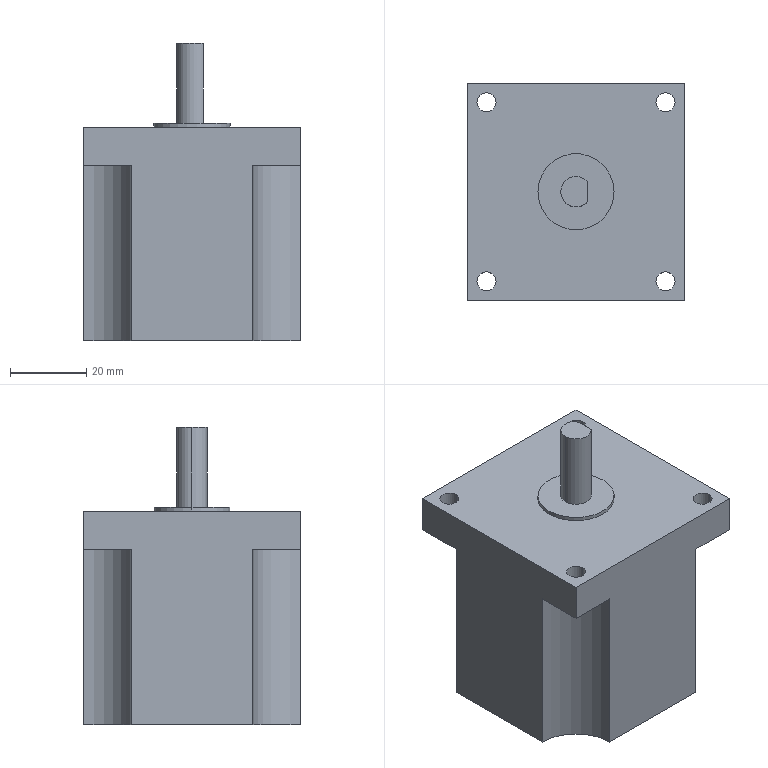Part | SolidWorks | features ICE 5, Extrusion 1 | 1 solid | 29 faces | box 57 x 57 x 78 mm | volume 159872 mm3 | cylinder 16 | plane 13 | commonest cylinder face diameters 5 x8 25 x4 8 x2 20 x2
STEP:
#1=CARTESIAN_POINT('',(-4.,0.,78.));
#2=VERTEX_POINT('',#1);
#3=CARTESIAN_POINT('',(3.,-2.646,78.));
#4=VERTEX_POINT('',#3);
#5=CARTESIAN_POINT('',(0.,0.,78.));
#6=DIRECTION('',(0.,0.,1.));
#7=DIRECTION('',(1.,0.,0.));
#8=AXIS2_PLACEMENT_3D('',#5,#6,#7);
#9=CIRCLE('',#8,4.);
#10=EDGE_CURVE('',#2,#4,#9,.T.);
#11=ORIENTED_EDGE('',*,*,#10,.F.);
#12=CARTESIAN_POINT('',(-4.,0.,57.));
#13=VERTEX_POINT('',#12);
#14=CARTESIAN_POINT('',(-4.,0.,78.));
#15=DIRECTION('',(0.,0.,-1.));
#16=VECTOR('',#15,1000.);
#17=LINE('',#14,#16);
#18=EDGE_CURVE('',#2,#13,#17,.T.);
#19=ORIENTED_EDGE('',*,*,#18,.T.);
#20=CARTESIAN_POINT('',(3.,-2.646,57.));
#21=VERTEX_POINT('',#20);
#22=CARTESIAN_POINT('',(0.,0.,57.));
#23=DIRECTION('',(0.,0.,1.));
#24=DIRECTION('',(1.,0.,0.));
#25=AXIS2_PLACEMENT_3D('',#22,#23,#24);
#26=CIRCLE('',#25,4.);
#27=EDGE_CURVE('',#13,#21,#26,.T.);
#28=ORIENTED_EDGE('',*,*,#27,.T.);
#29=CARTESIAN_POINT('',(3.,-2.646,57.));
#30=DIRECTION('',(0.,0.,1.));
#31=VECTOR('',#30,1000.);
#32=LINE('',#29,#31);
#33=EDGE_CURVE('',#21,#4,#32,.T.);
#34=ORIENTED_EDGE('',*,*,#33,.T.);
#35=EDGE_LOOP('',(#11,#19,#28,#34));
#36=FACE_OUTER_BOUND('',#35,.T.);
#37=CARTESIAN_POINT('',(0.,0.,78.));
#38=DIRECTION('',(0.,0.,-1.));
#39=DIRECTION('',(-1.,0.,0.));
#40=AXIS2_PLACEMENT_3D('',#37,#38,#39);
#41=CYLINDRICAL_SURFACE('',#40,4.);
#42=ADVANCED_FACE('',(#36),#41,.T.);
#43=CARTESIAN_POINT('',(10.,0.,57.));
#44=VERTEX_POINT('',#43);
#45=CARTESIAN_POINT('',(-10.,0.,57.));
#46=VERTEX_POINT('',#45);
#47=CARTESIAN_POINT('',(0.,0.,57.));
#48=DIRECTION('',(0.,0.,1.));
#49=DIRECTION('',(1.,0.,0.));
#50=AXIS2_PLACEMENT_3D('',#47,#48,#49);
#51=CIRCLE('',#50,10.);
#52=EDGE_CURVE('',#44,#46,#51,.T.);
#53=ORIENTED_EDGE('',*,*,#52,.F.);
#54=CARTESIAN_POINT('',(10.,0.,56.));
#55=VERTEX_POINT('',#54);
#56=CARTESIAN_POINT('',(10.,0.,57.));
#57=DIRECTION('',(0.,0.,-1.));
#58=VECTOR('',#57,1000.);
#59=LINE('',#56,#58);
#60=EDGE_CURVE('',#44,#55,#59,.T.);
#61=ORIENTED_EDGE('',*,*,#60,.T.);
#62=CARTESIAN_POINT('',(-10.,0.,56.));
#63=VERTEX_POINT('',#62);
#64=CARTESIAN_POINT('',(0.,0.,56.));
#65=DIRECTION('',(0.,0.,1.));
#66=DIRECTION('',(1.,0.,0.));
#67=AXIS2_PLACEMENT_3D('',#64,#65,#66);
#68=CIRCLE('',#67,10.);
#69=EDGE_CURVE('',#55,#63,#68,.T.);
#70=ORIENTED_EDGE('',*,*,#69,.T.);
#71=CARTESIAN_POINT('',(-10.,0.,57.));
#72=DIRECTION('',(0.,0.,-1.));
#73=VECTOR('',#72,1000.);
#74=LINE('',#71,#73);
#75=EDGE_CURVE('',#46,#63,#74,.T.);
#76=ORIENTED_EDGE('',*,*,#75,.F.);
#77=EDGE_LOOP('',(#53,#61,#70,#76));
#78=FACE_OUTER_BOUND('',#77,.T.);
#79=CARTESIAN_POINT('',(0.,0.,57.));
#80=DIRECTION('',(0.,0.,-1.));
#81=DIRECTION('',(-1.,0.,0.));
#82=AXIS2_PLACEMENT_3D('',#79,#80,#81);
#83=CYLINDRICAL_SURFACE('',#82,10.);
#84=ADVANCED_FACE('',(#78),#83,.T.);
#85=CARTESIAN_POINT('',(-21.,-23.5,46.));
#86=VERTEX_POINT('',#85);
#87=CARTESIAN_POINT('',(-26.,-23.5,46.));
#88=VERTEX_POINT('',#87);
#89=CARTESIAN_POINT('',(-23.5,-23.5,46.));
#90=DIRECTION('',(0.,0.,-1.));
#91=DIRECTION('',(1.,0.,0.));
#92=AXIS2_PLACEMENT_3D('',#89,#90,#91);
#93=CIRCLE('',#92,2.5);
#94=EDGE_CURVE('',#86,#88,#93,.T.);
#95=ORIENTED_EDGE('',*,*,#94,.T.);
#96=CARTESIAN_POINT('',(-26.,-23.5,56.));
#97=VERTEX_POINT('',#96);
#98=CARTESIAN_POINT('',(-26.,-23.5,-42.));
#99=DIRECTION('',(0.,0.,1.));
#100=VECTOR('',#99,1000.);
#101=LINE('',#98,#100);
#102=EDGE_CURVE('',#88,#97,#101,.T.);
#103=ORIENTED_EDGE('',*,*,#102,.T.);
#104=CARTESIAN_POINT('',(-21.,-23.5,56.));
#105=VERTEX_POINT('',#104);
#106=CARTESIAN_POINT('',(-23.5,-23.5,56.));
#107=DIRECTION('',(0.,0.,1.));
#108=DIRECTION('',(1.,0.,0.));
#109=AXIS2_PLACEMENT_3D('',#106,#107,#108);
#110=CIRCLE('',#109,2.5);
#111=EDGE_CURVE('',#97,#105,#110,.T.);
#112=ORIENTED_EDGE('',*,*,#111,.T.);
#113=CARTESIAN_POINT('',(-21.,-23.5,-42.));
#114=DIRECTION('',(0.,0.,1.));
#115=VECTOR('',#114,1000.);
#116=LINE('',#113,#115);
#117=EDGE_CURVE('',#86,#105,#116,.T.);
#118=ORIENTED_EDGE('',*,*,#117,.F.);
#119=EDGE_LOOP('',(#95,#103,#112,#118));
#120=FACE_OUTER_BOUND('',#119,.T.);
#121=CARTESIAN_POINT('',(-23.5,-23.5,-42.));
#122=DIRECTION('',(0.,0.,1.));
#123=DIRECTION('',(1.,0.,0.));
#124=AXIS2_PLACEMENT_3D('',#121,#122,#123);
#125=CYLINDRICAL_SURFACE('',#124,2.5);
#126=ADVANCED_FACE('',(#120),#125,.F.);
#127=CARTESIAN_POINT('',(26.,-23.5,46.));
#128=VERTEX_POINT('',#127);
#129=CARTESIAN_POINT('',(21.,-23.5,46.));
#130=VERTEX_POINT('',#129);
#131=CARTESIAN_POINT('',(23.5,-23.5,46.));
#132=DIRECTION('',(0.,0.,-1.));
#133=DIRECTION('',(1.,0.,0.));
#134=AXIS2_PLACEMENT_3D('',#131,#132,#133);
#135=CIRCLE('',#134,2.5);
#136=EDGE_CURVE('',#128,#130,#135,.T.);
#137=ORIENTED_EDGE('',*,*,#136,.T.);
#138=CARTESIAN_POINT('',(21.,-23.5,56.));
#139=VERTEX_POINT('',#138);
#140=CARTESIAN_POINT('',(21.,-23.5,-42.));
#141=DIRECTION('',(0.,0.,1.));
#142=VECTOR('',#141,1000.);
#143=LINE('',#140,#142);
#144=EDGE_CURVE('',#130,#139,#143,.T.);
#145=ORIENTED_EDGE('',*,*,#144,.T.);
#146=CARTESIAN_POINT('',(26.,-23.5,56.));
#147=VERTEX_POINT('',#146);
#148=CARTESIAN_POINT('',(23.5,-23.5,56.));
#149=DIRECTION('',(0.,0.,1.));
#150=DIRECTION('',(1.,0.,0.));
#151=AXIS2_PLACEMENT_3D('',#148,#149,#150);
#152=CIRCLE('',#151,2.5);
#153=EDGE_CURVE('',#139,#147,#152,.T.);
#154=ORIENTED_EDGE('',*,*,#153,.T.);
#155=CARTESIAN_POINT('',(26.,-23.5,-42.));
#156=DIRECTION('',(0.,0.,1.));
#157=VECTOR('',#156,1000.);
#158=LINE('',#155,#157);
#159=EDGE_CURVE('',#128,#147,#158,.T.);
#160=ORIENTED_EDGE('',*,*,#159,.F.);
#161=EDGE_LOOP('',(#137,#145,#154,#160));
#162=FACE_OUTER_BOUND('',#161,.T.);
#163=CARTESIAN_POINT('',(23.5,-23.5,-42.));
#164=DIRECTION('',(0.,0.,1.));
#165=DIRECTION('',(1.,0.,0.));
#166=AXIS2_PLACEMENT_3D('',#163,#164,#165);
#167=CYLINDRICAL_SURFACE('',#166,2.5);
#168=ADVANCED_FACE('',(#162),#167,.F.);
#169=CARTESIAN_POINT('',(26.,23.5,46.));
#170=VERTEX_POINT('',#169);
#171=CARTESIAN_POINT('',(21.,23.5,46.));
#172=VERTEX_POINT('',#171);
#173=CARTESIAN_POINT('',(23.5,23.5,46.));
#174=DIRECTION('',(0.,0.,-1.));
#175=DIRECTION('',(1.,0.,0.));
#176=AXIS2_PLACEMENT_3D('',#173,#174,#175);
#177=CIRCLE('',#176,2.5);
#178=EDGE_CURVE('',#170,#172,#177,.T.);
#179=ORIENTED_EDGE('',*,*,#178,.T.);
#180=CARTESIAN_POINT('',(21.,23.5,56.));
#181=VERTEX_POINT('',#180);
#182=CARTESIAN_POINT('',(21.,23.5,-42.));
#183=DIRECTION('',(0.,0.,1.));
#184=VECTOR('',#183,1000.);
#185=LINE('',#182,#184);
#186=EDGE_CURVE('',#172,#181,#185,.T.);
#187=ORIENTED_EDGE('',*,*,#186,.T.);
#188=CARTESIAN_POINT('',(26.,23.5,56.));
#189=VERTEX_POINT('',#188);
#190=CARTESIAN_POINT('',(23.5,23.5,56.));
#191=DIRECTION('',(0.,0.,1.));
#192=DIRECTION('',(1.,0.,0.));
#193=AXIS2_PLACEMENT_3D('',#190,#191,#192);
#194=CIRCLE('',#193,2.5);
#195=EDGE_CURVE('',#181,#189,#194,.T.);
#196=ORIENTED_EDGE('',*,*,#195,.T.);
#197=CARTESIAN_POINT('',(26.,23.5,-42.));
#198=DIRECTION('',(0.,0.,1.));
#199=VECTOR('',#198,1000.);
#200=LINE('',#197,#199);
#201=EDGE_CURVE('',#170,#189,#200,.T.);
#202=ORIENTED_EDGE('',*,*,#201,.F.);
#203=EDGE_LOOP('',(#179,#187,#196,#202));
#204=FACE_OUTER_BOUND('',#203,.T.);
#205=CARTESIAN_POINT('',(23.5,23.5,-42.));
#206=DIRECTION('',(0.,0.,1.));
#207=DIRECTION('',(1.,0.,0.));
#208=AXIS2_PLACEMENT_3D('',#205,#206,#207);
#209=CYLINDRICAL_SURFACE('',#208,2.5);
#210=ADVANCED_FACE('',(#204),#209,.F.);
#211=CARTESIAN_POINT('',(-21.,23.5,46.));
#212=VERTEX_POINT('',#211);
#213=CARTESIAN_POINT('',(-26.,23.5,46.));
#214=VERTEX_POINT('',#213);
#215=CARTESIAN_POINT('',(-23.5,23.5,46.));
#216=DIRECTION('',(0.,0.,-1.));
#217=DIRECTION('',(1.,0.,0.));
#218=AXIS2_PLACEMENT_3D('',#215,#216,#217);
#219=CIRCLE('',#218,2.5);
#220=EDGE_CURVE('',#212,#214,#219,.T.);
#221=ORIENTED_EDGE('',*,*,#220,.T.);
#222=CARTESIAN_POINT('',(-26.,23.5,56.));
#223=VERTEX_POINT('',#222);
#224=CARTESIAN_POINT('',(-26.,23.5,-42.));
#225=DIRECTION('',(0.,0.,1.));
#226=VECTOR('',#225,1000.);
#227=LINE('',#224,#226);
#228=EDGE_CURVE('',#214,#223,#227,.T.);
#229=ORIENTED_EDGE('',*,*,#228,.T.);
#230=CARTESIAN_POINT('',(-21.,23.5,56.));
#231=VERTEX_POINT('',#230);
#232=CARTESIAN_POINT('',(-23.5,23.5,56.));
#233=DIRECTION('',(0.,0.,1.));
#234=DIRECTION('',(1.,0.,0.));
#235=AXIS2_PLACEMENT_3D('',#232,#233,#234);
#236=CIRCLE('',#235,2.5);
#237=EDGE_CURVE('',#223,#231,#236,.T.);
#238=ORIENTED_EDGE('',*,*,#237,.T.);
#239=CARTESIAN_POINT('',(-21.,23.5,-42.));
#240=DIRECTION('',(0.,0.,1.));
#241=VECTOR('',#240,1000.);
#242=LINE('',#239,#241);
#243=EDGE_CURVE('',#212,#231,#242,.T.);
#244=ORIENTED_EDGE('',*,*,#243,.F.);
#245=EDGE_LOOP('',(#221,#229,#238,#244));
#246=FACE_OUTER_BOUND('',#245,.T.);
#247=CARTESIAN_POINT('',(-23.5,23.5,-42.));
#248=DIRECTION('',(0.,0.,1.));
#249=DIRECTION('',(1.,0.,0.));
#250=AXIS2_PLACEMENT_3D('',#247,#248,#249);
#251=CYLINDRICAL_SURFACE('',#250,2.5);
#252=ADVANCED_FACE('',(#246),#251,.F.);
#253=CARTESIAN_POINT('',(-28.5,-16.,0.));
#254=VERTEX_POINT('',#253);
#255=CARTESIAN_POINT('',(-28.5,-16.,46.));
#256=VERTEX_POINT('',#255);
#257=CARTESIAN_POINT('',(-28.5,-16.,91.355));
#258=DIRECTION('',(0.,0.,1.));
#259=VECTOR('',#258,1000.);
#260=LINE('',#257,#259);
#261=EDGE_CURVE('',#254,#256,#260,.T.);
#262=ORIENTED_EDGE('',*,*,#261,.T.);
#263=CARTESIAN_POINT('',(-28.5,-28.5,46.));
#264=VERTEX_POINT('',#263);
#265=CARTESIAN_POINT('',(-28.5,-28.5,46.));
#266=DIRECTION('',(0.,-1.,0.));
#267=VECTOR('',#266,1000.);
#268=LINE('',#265,#267);
#269=EDGE_CURVE('',#256,#264,#268,.T.);
#270=ORIENTED_EDGE('',*,*,#269,.T.);
#271=CARTESIAN_POINT('',(-28.5,-28.5,56.));
#272=VERTEX_POINT('',#271);
#273=CARTESIAN_POINT('',(-28.5,-28.5,56.));
#274=DIRECTION('',(0.,0.,-1.));
#275=VECTOR('',#274,1000.);
#276=LINE('',#273,#275);
#277=EDGE_CURVE('',#272,#264,#276,.T.);
#278=ORIENTED_EDGE('',*,*,#277,.F.);
#279=CARTESIAN_POINT('',(-28.5,28.5,56.));
#280=VERTEX_POINT('',#279);
#281=CARTESIAN_POINT('',(-28.5,-28.5,56.));
#282=DIRECTION('',(0.,-1.,0.));
#283=VECTOR('',#282,1000.);
#284=LINE('',#281,#283);
#285=EDGE_CURVE('',#280,#272,#284,.T.);
#286=ORIENTED_EDGE('',*,*,#285,.F.);
#287=CARTESIAN_POINT('',(-28.5,28.5,46.));
#288=VERTEX_POINT('',#287);
#289=CARTESIAN_POINT('',(-28.5,28.5,56.));
#290=DIRECTION('',(0.,0.,-1.));
#291=VECTOR('',#290,1000.);
#292=LINE('',#289,#291);
#293=EDGE_CURVE('',#280,#288,#292,.T.);
#294=ORIENTED_EDGE('',*,*,#293,.T.);
#295=CARTESIAN_POINT('',(-28.5,16.,46.));
#296=VERTEX_POINT('',#295);
#297=CARTESIAN_POINT('',(-28.5,-28.5,46.));
#298=DIRECTION('',(0.,-1.,0.));
#299=VECTOR('',#298,1000.);
#300=LINE('',#297,#299);
#301=EDGE_CURVE('',#288,#296,#300,.T.);
#302=ORIENTED_EDGE('',*,*,#301,.T.);
#303=CARTESIAN_POINT('',(-28.5,16.,0.));
#304=VERTEX_POINT('',#303);
#305=CARTESIAN_POINT('',(-28.5,16.,91.355));
#306=DIRECTION('',(0.,0.,-1.));
#307=VECTOR('',#306,1000.);
#308=LINE('',#305,#307);
#309=EDGE_CURVE('',#296,#304,#308,.T.);
#310=ORIENTED_EDGE('',*,*,#309,.T.);
#311=CARTESIAN_POINT('',(-28.5,-28.5,0.));
#312=DIRECTION('',(0.,-1.,0.));
#313=VECTOR('',#312,1000.);
#314=LINE('',#311,#313);
#315=EDGE_CURVE('',#304,#254,#314,.T.);
#316=ORIENTED_EDGE('',*,*,#315,.T.);
#317=EDGE_LOOP('',(#262,#270,#278,#286,#294,#302,#310,#316));
#318=FACE_OUTER_BOUND('',#317,.T.);
#319=CARTESIAN_POINT('',(-28.5,-28.5,56.));
#320=DIRECTION('',(1.,0.,0.));
#321=DIRECTION('',(0.,0.,-1.));
#322=AXIS2_PLACEMENT_3D('',#319,#320,#321);
#323=PLANE('',#322);
#324=ADVANCED_FACE('',(#318),#323,.F.);
#325=CARTESIAN_POINT('',(16.,-28.5,0.));
#326=VERTEX_POINT('',#325);
#327=CARTESIAN_POINT('',(16.,-28.5,46.));
#328=VERTEX_POINT('',#327);
#329=CARTESIAN_POINT('',(16.,-28.5,91.355));
#330=DIRECTION('',(0.,0.,1.));
#331=VECTOR('',#330,1000.);
#332=LINE('',#329,#331);
#333=EDGE_CURVE('',#326,#328,#332,.T.);
#334=ORIENTED_EDGE('',*,*,#333,.T.);
#335=CARTESIAN_POINT('',(28.5,-28.5,46.));
#336=VERTEX_POINT('',#335);
#337=CARTESIAN_POINT('',(28.5,-28.5,46.));
#338=DIRECTION('',(1.,0.,0.));
#339=VECTOR('',#338,1000.);
#340=LINE('',#337,#339);
#341=EDGE_CURVE('',#328,#336,#340,.T.);
#342=ORIENTED_EDGE('',*,*,#341,.T.);
#343=CARTESIAN_POINT('',(28.5,-28.5,56.));
#344=VERTEX_POINT('',#343);
#345=CARTESIAN_POINT('',(28.5,-28.5,56.));
#346=DIRECTION('',(0.,0.,-1.));
#347=VECTOR('',#346,1000.);
#348=LINE('',#345,#347);
#349=EDGE_CURVE('',#344,#336,#348,.T.);
#350=ORIENTED_EDGE('',*,*,#349,.F.);
#351=CARTESIAN_POINT('',(28.5,-28.5,56.));
#352=DIRECTION('',(1.,0.,0.));
#353=VECTOR('',#352,1000.);
#354=LINE('',#351,#353);
#355=EDGE_CURVE('',#272,#344,#354,.T.);
#356=ORIENTED_EDGE('',*,*,#355,.F.);
#357=ORIENTED_EDGE('',*,*,#277,.T.);
#358=CARTESIAN_POINT('',(-16.,-28.5,46.));
#359=VERTEX_POINT('',#358);
#360=CARTESIAN_POINT('',(28.5,-28.5,46.));
#361=DIRECTION('',(1.,0.,0.));
#362=VECTOR('',#361,1000.);
#363=LINE('',#360,#362);
#364=EDGE_CURVE('',#264,#359,#363,.T.);
#365=ORIENTED_EDGE('',*,*,#364,.T.);
#366=CARTESIAN_POINT('',(-16.,-28.5,0.));
#367=VERTEX_POINT('',#366);
#368=CARTESIAN_POINT('',(-16.,-28.5,91.355));
#369=DIRECTION('',(0.,0.,-1.));
#370=VECTOR('',#369,1000.);
#371=LINE('',#368,#370);
#372=EDGE_CURVE('',#359,#367,#371,.T.);
#373=ORIENTED_EDGE('',*,*,#372,.T.);
#374=CARTESIAN_POINT('',(28.5,-28.5,0.));
#375=DIRECTION('',(1.,0.,0.));
#376=VECTOR('',#375,1000.);
#377=LINE('',#374,#376);
#378=EDGE_CURVE('',#367,#326,#377,.T.);
#379=ORIENTED_EDGE('',*,*,#378,.T.);
#380=EDGE_LOOP('',(#334,#342,#350,#356,#357,#365,#373,#379));
#381=FACE_OUTER_BOUND('',#380,.T.);
#382=CARTESIAN_POINT('',(28.5,-28.5,56.));
#383=DIRECTION('',(0.,1.,0.));
#384=DIRECTION('',(-1.,0.,0.));
#385=AXIS2_PLACEMENT_3D('',#382,#383,#384);
#386=PLANE('',#385);
#387=ADVANCED_FACE('',(#381),#386,.F.);
#388=ORIENTED_EDGE('',*,*,#349,.T.);
#389=CARTESIAN_POINT('',(28.5,-16.,46.));
#390=VERTEX_POINT('',#389);
#391=CARTESIAN_POINT('',(28.5,-28.5,46.));
#392=DIRECTION('',(0.,1.,0.));
#393=VECTOR('',#392,1000.);
#394=LINE('',#391,#393);
#395=EDGE_CURVE('',#336,#390,#394,.T.);
#396=ORIENTED_EDGE('',*,*,#395,.T.);
#397=CARTESIAN_POINT('',(28.5,-16.,0.));
#398=VERTEX_POINT('',#397);
#399=CARTESIAN_POINT('',(28.5,-16.,91.355));
#400=DIRECTION('',(0.,0.,-1.));
#401=VECTOR('',#400,1000.);
#402=LINE('',#399,#401);
#403=EDGE_CURVE('',#390,#398,#402,.T.);
#404=ORIENTED_EDGE('',*,*,#403,.T.);
#405=CARTESIAN_POINT('',(28.5,16.,0.));
#406=VERTEX_POINT('',#405);
#407=CARTESIAN_POINT('',(28.5,-28.5,0.));
#408=DIRECTION('',(0.,1.,0.));
#409=VECTOR('',#408,1000.);
#410=LINE('',#407,#409);
#411=EDGE_CURVE('',#398,#406,#410,.T.);
#412=ORIENTED_EDGE('',*,*,#411,.T.);
#413=CARTESIAN_POINT('',(28.5,16.,46.));
#414=VERTEX_POINT('',#413);
#415=CARTESIAN_POINT('',(28.5,16.,91.355));
#416=DIRECTION('',(0.,0.,1.));
#417=VECTOR('',#416,1000.);
#418=LINE('',#415,#417);
#419=EDGE_CURVE('',#406,#414,#418,.T.);
#420=ORIENTED_EDGE('',*,*,#419,.T.);
#421=CARTESIAN_POINT('',(28.5,28.5,46.));
#422=VERTEX_POINT('',#421);
#423=CARTESIAN_POINT('',(28.5,-28.5,46.));
#424=DIRECTION('',(0.,1.,0.));
#425=VECTOR('',#424,1000.);
#426=LINE('',#423,#425);
#427=EDGE_CURVE('',#414,#422,#426,.T.);
#428=ORIENTED_EDGE('',*,*,#427,.T.);
#429=CARTESIAN_POINT('',(28.5,28.5,56.));
#430=VERTEX_POINT('',#429);
#431=CARTESIAN_POINT('',(28.5,28.5,56.));
#432=DIRECTION('',(0.,0.,-1.));
#433=VECTOR('',#432,1000.);
#434=LINE('',#431,#433);
#435=EDGE_CURVE('',#430,#422,#434,.T.);
#436=ORIENTED_EDGE('',*,*,#435,.F.);
#437=CARTESIAN_POINT('',(28.5,-28.5,56.));
#438=DIRECTION('',(0.,1.,0.));
#439=VECTOR('',#438,1000.);
#440=LINE('',#437,#439);
#441=EDGE_CURVE('',#344,#430,#440,.T.);
#442=ORIENTED_EDGE('',*,*,#441,.F.);
#443=EDGE_LOOP('',(#388,#396,#404,#412,#420,#428,#436,#442));
#444=FACE_OUTER_BOUND('',#443,.T.);
#445=CARTESIAN_POINT('',(28.5,-28.5,56.));
#446=DIRECTION('',(-1.,0.,0.));
#447=DIRECTION('',(0.,0.,1.));
#448=AXIS2_PLACEMENT_3D('',#445,#446,#447);
#449=PLANE('',#448);
#450=ADVANCED_FACE('',(#444),#449,.F.);
#451=CARTESIAN_POINT('',(-16.,28.5,0.));
#452=VERTEX_POINT('',#451);
#453=CARTESIAN_POINT('',(-16.,28.5,46.));
#454=VERTEX_POINT('',#453);
#455=CARTESIAN_POINT('',(-16.,28.5,91.355));
#456=DIRECTION('',(0.,0.,1.));
#457=VECTOR('',#456,1000.);
#458=LINE('',#455,#457);
#459=EDGE_CURVE('',#452,#454,#458,.T.);
#460=ORIENTED_EDGE('',*,*,#459,.T.);
#461=CARTESIAN_POINT('',(28.5,28.5,46.));
#462=DIRECTION('',(-1.,0.,0.));
#463=VECTOR('',#462,1000.);
#464=LINE('',#461,#463);
#465=EDGE_CURVE('',#454,#288,#464,.T.);
#466=ORIENTED_EDGE('',*,*,#465,.T.);
#467=ORIENTED_EDGE('',*,*,#293,.F.);
#468=CARTESIAN_POINT('',(28.5,28.5,56.));
#469=DIRECTION('',(-1.,0.,0.));
#470=VECTOR('',#469,1000.);
#471=LINE('',#468,#470);
#472=EDGE_CURVE('',#430,#280,#471,.T.);
#473=ORIENTED_EDGE('',*,*,#472,.F.);
#474=ORIENTED_EDGE('',*,*,#435,.T.);
#475=CARTESIAN_POINT('',(16.,28.5,46.));
#476=VERTEX_POINT('',#475);
#477=CARTESIAN_POINT('',(28.5,28.5,46.));
#478=DIRECTION('',(-1.,0.,0.));
#479=VECTOR('',#478,1000.);
#480=LINE('',#477,#479);
#481=EDGE_CURVE('',#422,#476,#480,.T.);
#482=ORIENTED_EDGE('',*,*,#481,.T.);
#483=CARTESIAN_POINT('',(16.,28.5,0.));
#484=VERTEX_POINT('',#483);
#485=CARTESIAN_POINT('',(16.,28.5,91.355));
#486=DIRECTION('',(0.,0.,-1.));
#487=VECTOR('',#486,1000.);
#488=LINE('',#485,#487);
#489=EDGE_CURVE('',#476,#484,#488,.T.);
#490=ORIENTED_EDGE('',*,*,#489,.T.);
#491=CARTESIAN_POINT('',(28.5,28.5,0.));
#492=DIRECTION('',(-1.,0.,0.));
#493=VECTOR('',#492,1000.);
#494=LINE('',#491,#493);
#495=EDGE_CURVE('',#484,#452,#494,.T.);
#496=ORIENTED_EDGE('',*,*,#495,.T.);
#497=EDGE_LOOP('',(#460,#466,#467,#473,#474,#482,#490,#496));
#498=FACE_OUTER_BOUND('',#497,.T.);
#499=CARTESIAN_POINT('',(28.5,28.5,56.));
#500=DIRECTION('',(0.,-1.,0.));
#501=DIRECTION('',(1.,0.,0.));
#502=AXIS2_PLACEMENT_3D('',#499,#500,#501);
#503=PLANE('',#502);
#504=ADVANCED_FACE('',(#498),#503,.F.);
#505=CARTESIAN_POINT('',(0.,0.,56.));
#506=DIRECTION('',(0.,0.,1.));
#507=DIRECTION('',(1.,0.,0.));
#508=AXIS2_PLACEMENT_3D('',#505,#506,#507);
#509=CIRCLE('',#508,10.);
#510=EDGE_CURVE('',#63,#55,#509,.T.);
#511=ORIENTED_EDGE('',*,*,#510,.F.);
#512=ORIENTED_EDGE('',*,*,#69,.F.);
#513=EDGE_LOOP('',(#511,#512));
#514=FACE_BOUND('',#513,.T.);
#515=CARTESIAN_POINT('',(-23.5,-23.5,56.));
#516=DIRECTION('',(0.,0.,1.));
#517=DIRECTION('',(1.,0.,0.));
#518=AXIS2_PLACEMENT_3D('',#515,#516,#517);
#519=CIRCLE('',#518,2.5);
#520=EDGE_CURVE('',#105,#97,#519,.T.);
#521=ORIENTED_EDGE('',*,*,#520,.F.);
#522=ORIENTED_EDGE('',*,*,#111,.F.);
#523=EDGE_LOOP('',(#521,#522));
#524=FACE_BOUND('',#523,.T.);
#525=CARTESIAN_POINT('',(23.5,-23.5,56.));
#526=DIRECTION('',(0.,0.,1.));
#527=DIRECTION('',(1.,0.,0.));
#528=AXIS2_PLACEMENT_3D('',#525,#526,#527);
#529=CIRCLE('',#528,2.5);
#530=EDGE_CURVE('',#147,#139,#529,.T.);
#531=ORIENTED_EDGE('',*,*,#530,.F.);
#532=ORIENTED_EDGE('',*,*,#153,.F.);
#533=EDGE_LOOP('',(#531,#532));
#534=FACE_BOUND('',#533,.T.);
#535=CARTESIAN_POINT('',(23.5,23.5,56.));
#536=DIRECTION('',(0.,0.,1.));
#537=DIRECTION('',(1.,0.,0.));
#538=AXIS2_PLACEMENT_3D('',#535,#536,#537);
#539=CIRCLE('',#538,2.5);
#540=EDGE_CURVE('',#189,#181,#539,.T.);
#541=ORIENTED_EDGE('',*,*,#540,.F.);
#542=ORIENTED_EDGE('',*,*,#195,.F.);
#543=EDGE_LOOP('',(#541,#542));
#544=FACE_BOUND('',#543,.T.);
#545=CARTESIAN_POINT('',(-23.5,23.5,56.));
#546=DIRECTION('',(0.,0.,1.));
#547=DIRECTION('',(1.,0.,0.));
#548=AXIS2_PLACEMENT_3D('',#545,#546,#547);
#549=CIRCLE('',#548,2.5);
#550=EDGE_CURVE('',#231,#223,#549,.T.);
#551=ORIENTED_EDGE('',*,*,#550,.F.);
#552=ORIENTED_EDGE('',*,*,#237,.F.);
#553=EDGE_LOOP('',(#551,#552));
#554=FACE_BOUND('',#553,.T.);
#555=ORIENTED_EDGE('',*,*,#285,.T.);
#556=ORIENTED_EDGE('',*,*,#355,.T.);
#557=ORIENTED_EDGE('',*,*,#441,.T.);
#558=ORIENTED_EDGE('',*,*,#472,.T.);
#559=EDGE_LOOP('',(#555,#556,#557,#558));
#560=FACE_OUTER_BOUND('',#559,.T.);
#561=CARTESIAN_POINT('',(0.,0.,56.));
#562=DIRECTION('',(0.,0.,1.));
#563=DIRECTION('',(1.,0.,0.));
#564=AXIS2_PLACEMENT_3D('',#561,#562,#563);
#565=PLANE('',#564);
#566=ADVANCED_FACE('',(#514,#524,#534,#544,#554,#560),#565,.T.);
#567=ORIENTED_EDGE('',*,*,#411,.F.);
#568=CARTESIAN_POINT('',(28.5,-28.5,0.));
#569=DIRECTION('',(0.,0.,-1.));
#570=DIRECTION('',(-1.,0.,0.));
#571=AXIS2_PLACEMENT_3D('',#568,#569,#570);
#572=CIRCLE('',#571,12.5);
#573=EDGE_CURVE('',#326,#398,#572,.T.);
#574=ORIENTED_EDGE('',*,*,#573,.F.);
#575=ORIENTED_EDGE('',*,*,#378,.F.);
#576=CARTESIAN_POINT('',(-28.5,-28.5,0.));
#577=DIRECTION('',(0.,0.,-1.));
#578=DIRECTION('',(-1.,0.,0.));
#579=AXIS2_PLACEMENT_3D('',#576,#577,#578);
#580=CIRCLE('',#579,12.5);
#581=EDGE_CURVE('',#254,#367,#580,.T.);
#582=ORIENTED_EDGE('',*,*,#581,.F.);
#583=ORIENTED_EDGE('',*,*,#315,.F.);
#584=CARTESIAN_POINT('',(-28.5,28.5,0.));
#585=DIRECTION('',(0.,0.,-1.));
#586=DIRECTION('',(-1.,0.,0.));
#587=AXIS2_PLACEMENT_3D('',#584,#585,#586);
#588=CIRCLE('',#587,12.5);
#589=EDGE_CURVE('',#452,#304,#588,.T.);
#590=ORIENTED_EDGE('',*,*,#589,.F.);
#591=ORIENTED_EDGE('',*,*,#495,.F.);
#592=CARTESIAN_POINT('',(28.5,28.5,0.));
#593=DIRECTION('',(0.,0.,-1.));
#594=DIRECTION('',(-1.,0.,0.));
#595=AXIS2_PLACEMENT_3D('',#592,#593,#594);
#596=CIRCLE('',#595,12.5);
#597=EDGE_CURVE('',#406,#484,#596,.T.);
#598=ORIENTED_EDGE('',*,*,#597,.F.);
#599=EDGE_LOOP('',(#567,#574,#575,#582,#583,#590,#591,#598));
#600=FACE_OUTER_BOUND('',#599,.T.);
#601=CARTESIAN_POINT('',(0.,0.,0.));
#602=DIRECTION('',(0.,0.,1.));
#603=DIRECTION('',(1.,0.,0.));
#604=AXIS2_PLACEMENT_3D('',#601,#602,#603);
#605=PLANE('',#604);
#606=ADVANCED_FACE('',(#600),#605,.F.);
#607=ORIENTED_EDGE('',*,*,#228,.F.);
#608=CARTESIAN_POINT('',(-23.5,23.5,46.));
#609=DIRECTION('',(0.,0.,-1.));
#610=DIRECTION('',(1.,0.,0.));
#611=AXIS2_PLACEMENT_3D('',#608,#609,#610);
#612=CIRCLE('',#611,2.5);
#613=EDGE_CURVE('',#214,#212,#612,.T.);
#614=ORIENTED_EDGE('',*,*,#613,.T.);
#615=ORIENTED_EDGE('',*,*,#243,.T.);
#616=ORIENTED_EDGE('',*,*,#550,.T.);
#617=EDGE_LOOP('',(#607,#614,#615,#616));
#618=FACE_OUTER_BOUND('',#617,.T.);
#619=CARTESIAN_POINT('',(-23.5,23.5,-42.));
#620=DIRECTION('',(0.,0.,1.));
#621=DIRECTION('',(1.,0.,0.));
#622=AXIS2_PLACEMENT_3D('',#619,#620,#621);
#623=CYLINDRICAL_SURFACE('',#622,2.5);
#624=ADVANCED_FACE('',(#618),#623,.F.);
#625=ORIENTED_EDGE('',*,*,#186,.F.);
#626=CARTESIAN_POINT('',(23.5,23.5,46.));
#627=DIRECTION('',(0.,0.,-1.));
#628=DIRECTION('',(1.,0.,0.));
#629=AXIS2_PLACEMENT_3D('',#626,#627,#628);
#630=CIRCLE('',#629,2.5);
#631=EDGE_CURVE('',#172,#170,#630,.T.);
#632=ORIENTED_EDGE('',*,*,#631,.T.);
#633=ORIENTED_EDGE('',*,*,#201,.T.);
#634=ORIENTED_EDGE('',*,*,#540,.T.);
#635=EDGE_LOOP('',(#625,#632,#633,#634));
#636=FACE_OUTER_BOUND('',#635,.T.);
#637=CARTESIAN_POINT('',(23.5,23.5,-42.));
#638=DIRECTION('',(0.,0.,1.));
#639=DIRECTION('',(1.,0.,0.));
#640=AXIS2_PLACEMENT_3D('',#637,#638,#639);
#641=CYLINDRICAL_SURFACE('',#640,2.5);
#642=ADVANCED_FACE('',(#636),#641,.F.);
#643=ORIENTED_EDGE('',*,*,#144,.F.);
#644=CARTESIAN_POINT('',(23.5,-23.5,46.));
#645=DIRECTION('',(0.,0.,-1.));
#646=DIRECTION('',(1.,0.,0.));
#647=AXIS2_PLACEMENT_3D('',#644,#645,#646);
#648=CIRCLE('',#647,2.5);
#649=EDGE_CURVE('',#130,#128,#648,.T.);
#650=ORIENTED_EDGE('',*,*,#649,.T.);
#651=ORIENTED_EDGE('',*,*,#159,.T.);
#652=ORIENTED_EDGE('',*,*,#530,.T.);
#653=EDGE_LOOP('',(#643,#650,#651,#652));
#654=FACE_OUTER_BOUND('',#653,.T.);
#655=CARTESIAN_POINT('',(23.5,-23.5,-42.));
#656=DIRECTION('',(0.,0.,1.));
#657=DIRECTION('',(1.,0.,0.));
#658=AXIS2_PLACEMENT_3D('',#655,#656,#657);
#659=CYLINDRICAL_SURFACE('',#658,2.5);
#660=ADVANCED_FACE('',(#654),#659,.F.);
#661=ORIENTED_EDGE('',*,*,#102,.F.);
#662=CARTESIAN_POINT('',(-23.5,-23.5,46.));
#663=DIRECTION('',(0.,0.,-1.));
#664=DIRECTION('',(1.,0.,0.));
#665=AXIS2_PLACEMENT_3D('',#662,#663,#664);
#666=CIRCLE('',#665,2.5);
#667=EDGE_CURVE('',#88,#86,#666,.T.);
#668=ORIENTED_EDGE('',*,*,#667,.T.);
#669=ORIENTED_EDGE('',*,*,#117,.T.);
#670=ORIENTED_EDGE('',*,*,#520,.T.);
#671=EDGE_LOOP('',(#661,#668,#669,#670));
#672=FACE_OUTER_BOUND('',#671,.T.);
#673=CARTESIAN_POINT('',(-23.5,-23.5,-42.));
#674=DIRECTION('',(0.,0.,1.));
#675=DIRECTION('',(1.,0.,0.));
#676=AXIS2_PLACEMENT_3D('',#673,#674,#675);
#677=CYLINDRICAL_SURFACE('',#676,2.5);
#678=ADVANCED_FACE('',(#672),#677,.F.);
#679=ORIENTED_EDGE('',*,*,#60,.F.);
#680=CARTESIAN_POINT('',(0.,0.,57.));
#681=DIRECTION('',(0.,0.,1.));
#682=DIRECTION('',(1.,0.,0.));
#683=AXIS2_PLACEMENT_3D('',#680,#681,#682);
#684=CIRCLE('',#683,10.);
#685=EDGE_CURVE('',#46,#44,#684,.T.);
#686=ORIENTED_EDGE('',*,*,#685,.F.);
#687=ORIENTED_EDGE('',*,*,#75,.T.);
#688=ORIENTED_EDGE('',*,*,#510,.T.);
#689=EDGE_LOOP('',(#679,#686,#687,#688));
#690=FACE_OUTER_BOUND('',#689,.T.);
#691=CARTESIAN_POINT('',(0.,0.,57.));
#692=DIRECTION('',(0.,0.,-1.));
#693=DIRECTION('',(-1.,0.,0.));
#694=AXIS2_PLACEMENT_3D('',#691,#692,#693);
#695=CYLINDRICAL_SURFACE('',#694,10.);
#696=ADVANCED_FACE('',(#690),#695,.T.);
#697=CARTESIAN_POINT('',(3.,2.646,57.));
#698=VERTEX_POINT('',#697);
#699=CARTESIAN_POINT('',(0.,0.,57.));
#700=DIRECTION('',(0.,0.,1.));
#701=DIRECTION('',(1.,0.,0.));
#702=AXIS2_PLACEMENT_3D('',#699,#700,#701);
#703=CIRCLE('',#702,4.);
#704=EDGE_CURVE('',#698,#13,#703,.T.);
#705=ORIENTED_EDGE('',*,*,#704,.F.);
#706=CARTESIAN_POINT('',(3.,0.,57.));
#707=DIRECTION('',(0.,-1.,0.));
#708=VECTOR('',#707,1000.);
#709=LINE('',#706,#708);
#710=EDGE_CURVE('',#698,#21,#709,.T.);
#711=ORIENTED_EDGE('',*,*,#710,.T.);
#712=ORIENTED_EDGE('',*,*,#27,.F.);
#713=EDGE_LOOP('',(#705,#711,#712));
#714=FACE_BOUND('',#713,.T.);
#715=ORIENTED_EDGE('',*,*,#685,.T.);
#716=ORIENTED_EDGE('',*,*,#52,.T.);
#717=EDGE_LOOP('',(#715,#716));
#718=FACE_OUTER_BOUND('',#717,.T.);
#719=CARTESIAN_POINT('',(0.,0.,57.));
#720=DIRECTION('',(0.,0.,1.));
#721=DIRECTION('',(1.,0.,0.));
#722=AXIS2_PLACEMENT_3D('',#719,#720,#721);
#723=PLANE('',#722);
#724=ADVANCED_FACE('',(#714,#718),#723,.T.);
#725=ORIENTED_EDGE('',*,*,#18,.F.);
#726=CARTESIAN_POINT('',(3.,2.646,78.));
#727=VERTEX_POINT('',#726);
#728=CARTESIAN_POINT('',(0.,0.,78.));
#729=DIRECTION('',(0.,0.,1.));
#730=DIRECTION('',(1.,0.,0.));
#731=AXIS2_PLACEMENT_3D('',#728,#729,#730);
#732=CIRCLE('',#731,4.);
#733=EDGE_CURVE('',#727,#2,#732,.T.);
#734=ORIENTED_EDGE('',*,*,#733,.F.);
#735=CARTESIAN_POINT('',(3.,2.646,57.));
#736=DIRECTION('',(0.,0.,1.));
#737=VECTOR('',#736,1000.);
#738=LINE('',#735,#737);
#739=EDGE_CURVE('',#698,#727,#738,.T.);
#740=ORIENTED_EDGE('',*,*,#739,.F.);
#741=ORIENTED_EDGE('',*,*,#704,.T.);
#742=EDGE_LOOP('',(#725,#734,#740,#741));
#743=FACE_OUTER_BOUND('',#742,.T.);
#744=CARTESIAN_POINT('',(0.,0.,78.));
#745=DIRECTION('',(0.,0.,-1.));
#746=DIRECTION('',(-1.,0.,0.));
#747=AXIS2_PLACEMENT_3D('',#744,#745,#746);
#748=CYLINDRICAL_SURFACE('',#747,4.);
#749=ADVANCED_FACE('',(#743),#748,.T.);
#750=CARTESIAN_POINT('',(3.,0.,78.));
#751=DIRECTION('',(0.,-1.,0.));
#752=VECTOR('',#751,1000.);
#753=LINE('',#750,#752);
#754=EDGE_CURVE('',#727,#4,#753,.T.);
#755=ORIENTED_EDGE('',*,*,#754,.F.);
#756=ORIENTED_EDGE('',*,*,#733,.T.);
#757=ORIENTED_EDGE('',*,*,#10,.T.);
#758=EDGE_LOOP('',(#755,#756,#757));
#759=FACE_OUTER_BOUND('',#758,.T.);
#760=CARTESIAN_POINT('',(0.,0.,78.));
#761=DIRECTION('',(0.,0.,1.));
#762=DIRECTION('',(1.,0.,0.));
#763=AXIS2_PLACEMENT_3D('',#760,#761,#762);
#764=PLANE('',#763);
#765=ADVANCED_FACE('',(#759),#764,.T.);
#766=ORIENTED_EDGE('',*,*,#754,.T.);
#767=ORIENTED_EDGE('',*,*,#33,.F.);
#768=ORIENTED_EDGE('',*,*,#710,.F.);
#769=ORIENTED_EDGE('',*,*,#739,.T.);
#770=EDGE_LOOP('',(#766,#767,#768,#769));
#771=FACE_OUTER_BOUND('',#770,.T.);
#772=CARTESIAN_POINT('',(3.,0.,57.));
#773=DIRECTION('',(-1.,0.,0.));
#774=DIRECTION('',(0.,0.,1.));
#775=AXIS2_PLACEMENT_3D('',#772,#773,#774);
#776=PLANE('',#775);
#777=ADVANCED_FACE('',(#771),#776,.F.);
#778=ORIENTED_EDGE('',*,*,#581,.T.);
#779=ORIENTED_EDGE('',*,*,#372,.F.);
#780=CARTESIAN_POINT('',(-28.5,-28.5,46.));
#781=DIRECTION('',(0.,0.,-1.));
#782=DIRECTION('',(1.,0.,0.));
#783=AXIS2_PLACEMENT_3D('',#780,#781,#782);
#784=CIRCLE('',#783,12.5);
#785=EDGE_CURVE('',#256,#359,#784,.T.);
#786=ORIENTED_EDGE('',*,*,#785,.F.);
#787=ORIENTED_EDGE('',*,*,#261,.F.);
#788=EDGE_LOOP('',(#778,#779,#786,#787));
#789=FACE_OUTER_BOUND('',#788,.T.);
#790=CARTESIAN_POINT('',(-28.5,-28.5,91.355));
#791=DIRECTION('',(0.,0.,-1.));
#792=DIRECTION('',(-1.,0.,0.));
#793=AXIS2_PLACEMENT_3D('',#790,#791,#792);
#794=CYLINDRICAL_SURFACE('',#793,12.5);
#795=ADVANCED_FACE('',(#789),#794,.F.);
#796=ORIENTED_EDGE('',*,*,#94,.F.);
#797=ORIENTED_EDGE('',*,*,#667,.F.);
#798=EDGE_LOOP('',(#796,#797));
#799=FACE_BOUND('',#798,.T.);
#800=ORIENTED_EDGE('',*,*,#785,.T.);
#801=ORIENTED_EDGE('',*,*,#364,.F.);
#802=ORIENTED_EDGE('',*,*,#269,.F.);
#803=EDGE_LOOP('',(#800,#801,#802));
#804=FACE_OUTER_BOUND('',#803,.T.);
#805=CARTESIAN_POINT('',(0.,0.,46.));
#806=DIRECTION('',(0.,0.,1.));
#807=DIRECTION('',(1.,0.,0.));
#808=AXIS2_PLACEMENT_3D('',#805,#806,#807);
#809=PLANE('',#808);
#810=ADVANCED_FACE('',(#799,#804),#809,.F.);
#811=ORIENTED_EDGE('',*,*,#573,.T.);
#812=ORIENTED_EDGE('',*,*,#403,.F.);
#813=CARTESIAN_POINT('',(28.5,-28.5,46.));
#814=DIRECTION('',(0.,0.,-1.));
#815=DIRECTION('',(1.,0.,0.));
#816=AXIS2_PLACEMENT_3D('',#813,#814,#815);
#817=CIRCLE('',#816,12.5);
#818=EDGE_CURVE('',#328,#390,#817,.T.);
#819=ORIENTED_EDGE('',*,*,#818,.F.);
#820=ORIENTED_EDGE('',*,*,#333,.F.);
#821=EDGE_LOOP('',(#811,#812,#819,#820));
#822=FACE_OUTER_BOUND('',#821,.T.);
#823=CARTESIAN_POINT('',(28.5,-28.5,91.355));
#824=DIRECTION('',(0.,0.,-1.));
#825=DIRECTION('',(-1.,0.,0.));
#826=AXIS2_PLACEMENT_3D('',#823,#824,#825);
#827=CYLINDRICAL_SURFACE('',#826,12.5);
#828=ADVANCED_FACE('',(#822),#827,.F.);
#829=ORIENTED_EDGE('',*,*,#136,.F.);
#830=ORIENTED_EDGE('',*,*,#649,.F.);
#831=EDGE_LOOP('',(#829,#830));
#832=FACE_BOUND('',#831,.T.);
#833=ORIENTED_EDGE('',*,*,#818,.T.);
#834=ORIENTED_EDGE('',*,*,#395,.F.);
#835=ORIENTED_EDGE('',*,*,#341,.F.);
#836=EDGE_LOOP('',(#833,#834,#835));
#837=FACE_OUTER_BOUND('',#836,.T.);
#838=CARTESIAN_POINT('',(0.,0.,46.));
#839=DIRECTION('',(0.,0.,1.));
#840=DIRECTION('',(1.,0.,0.));
#841=AXIS2_PLACEMENT_3D('',#838,#839,#840);
#842=PLANE('',#841);
#843=ADVANCED_FACE('',(#832,#837),#842,.F.);
#844=ORIENTED_EDGE('',*,*,#597,.T.);
#845=ORIENTED_EDGE('',*,*,#489,.F.);
#846=CARTESIAN_POINT('',(28.5,28.5,46.));
#847=DIRECTION('',(0.,0.,-1.));
#848=DIRECTION('',(1.,0.,0.));
#849=AXIS2_PLACEMENT_3D('',#846,#847,#848);
#850=CIRCLE('',#849,12.5);
#851=EDGE_CURVE('',#414,#476,#850,.T.);
#852=ORIENTED_EDGE('',*,*,#851,.F.);
#853=ORIENTED_EDGE('',*,*,#419,.F.);
#854=EDGE_LOOP('',(#844,#845,#852,#853));
#855=FACE_OUTER_BOUND('',#854,.T.);
#856=CARTESIAN_POINT('',(28.5,28.5,91.355));
#857=DIRECTION('',(0.,0.,-1.));
#858=DIRECTION('',(-1.,0.,0.));
#859=AXIS2_PLACEMENT_3D('',#856,#857,#858);
#860=CYLINDRICAL_SURFACE('',#859,12.5);
#861=ADVANCED_FACE('',(#855),#860,.F.);
#862=ORIENTED_EDGE('',*,*,#178,.F.);
#863=ORIENTED_EDGE('',*,*,#631,.F.);
#864=EDGE_LOOP('',(#862,#863));
#865=FACE_BOUND('',#864,.T.);
#866=ORIENTED_EDGE('',*,*,#851,.T.);
#867=ORIENTED_EDGE('',*,*,#481,.F.);
#868=ORIENTED_EDGE('',*,*,#427,.F.);
#869=EDGE_LOOP('',(#866,#867,#868));
#870=FACE_OUTER_BOUND('',#869,.T.);
#871=CARTESIAN_POINT('',(0.,0.,46.));
#872=DIRECTION('',(0.,0.,1.));
#873=DIRECTION('',(1.,0.,0.));
#874=AXIS2_PLACEMENT_3D('',#871,#872,#873);
#875=PLANE('',#874);
#876=ADVANCED_FACE('',(#865,#870),#875,.F.);
#877=CARTESIAN_POINT('',(-28.5,28.5,46.));
#878=DIRECTION('',(0.,0.,-1.));
#879=DIRECTION('',(1.,0.,0.));
#880=AXIS2_PLACEMENT_3D('',#877,#878,#879);
#881=CIRCLE('',#880,12.5);
#882=EDGE_CURVE('',#454,#296,#881,.T.);
#883=ORIENTED_EDGE('',*,*,#882,.F.);
#884=ORIENTED_EDGE('',*,*,#459,.F.);
#885=ORIENTED_EDGE('',*,*,#589,.T.);
#886=ORIENTED_EDGE('',*,*,#309,.F.);
#887=EDGE_LOOP('',(#883,#884,#885,#886));
#888=FACE_OUTER_BOUND('',#887,.T.);
#889=CARTESIAN_POINT('',(-28.5,28.5,91.355));
#890=DIRECTION('',(0.,0.,-1.));
#891=DIRECTION('',(-1.,0.,0.));
#892=AXIS2_PLACEMENT_3D('',#889,#890,#891);
#893=CYLINDRICAL_SURFACE('',#892,12.5);
#894=ADVANCED_FACE('',(#888),#893,.F.);
#895=ORIENTED_EDGE('',*,*,#220,.F.);
#896=ORIENTED_EDGE('',*,*,#613,.F.);
#897=EDGE_LOOP('',(#895,#896));
#898=FACE_BOUND('',#897,.T.);
#899=ORIENTED_EDGE('',*,*,#465,.F.);
#900=ORIENTED_EDGE('',*,*,#882,.T.);
#901=ORIENTED_EDGE('',*,*,#301,.F.);
#902=EDGE_LOOP('',(#899,#900,#901));
#903=FACE_OUTER_BOUND('',#902,.T.);
#904=CARTESIAN_POINT('',(0.,0.,46.));
#905=DIRECTION('',(0.,0.,1.));
#906=DIRECTION('',(1.,0.,0.));
#907=AXIS2_PLACEMENT_3D('',#904,#905,#906);
#908=PLANE('',#907);
#909=ADVANCED_FACE('',(#898,#903),#908,.F.);
#910=CLOSED_SHELL('',(#42,#84,#126,#168,#210,#252,#324,#387,#450,#504,#566,#606,#624,#642,#660,#678,#696,#724,#749,#765,#777,#795,#810,#828,#843,#861,#876,#894,#909));
#911=MANIFOLD_SOLID_BREP('',#910);
#912=CARTESIAN_POINT('',(0.,0.,0.));
#913=DIRECTION('',(0.,0.,1.));
#914=DIRECTION('',(1.,0.,0.));
#915=AXIS2_PLACEMENT_3D('',#912,#913,#914);
#916=(LENGTH_UNIT()NAMED_UNIT(*)SI_UNIT(.MILLI.,.METRE.));
#917=UNCERTAINTY_MEASURE_WITH_UNIT(LENGTH_MEASURE(0.00001),#916,'','');
#918=(NAMED_UNIT(*)PLANE_ANGLE_UNIT()SI_UNIT($,.RADIAN.));
#919=(NAMED_UNIT(*)SI_UNIT($,.STERADIAN.)SOLID_ANGLE_UNIT());
#920=(GEOMETRIC_REPRESENTATION_CONTEXT(3)GLOBAL_UNCERTAINTY_ASSIGNED_CONTEXT((#917))GLOBAL_UNIT_ASSIGNED_CONTEXT((#916,#918,#919))REPRESENTATION_CONTEXT('',''));
#921=ADVANCED_BREP_SHAPE_REPRESENTATION('',(#911,#915),#920);